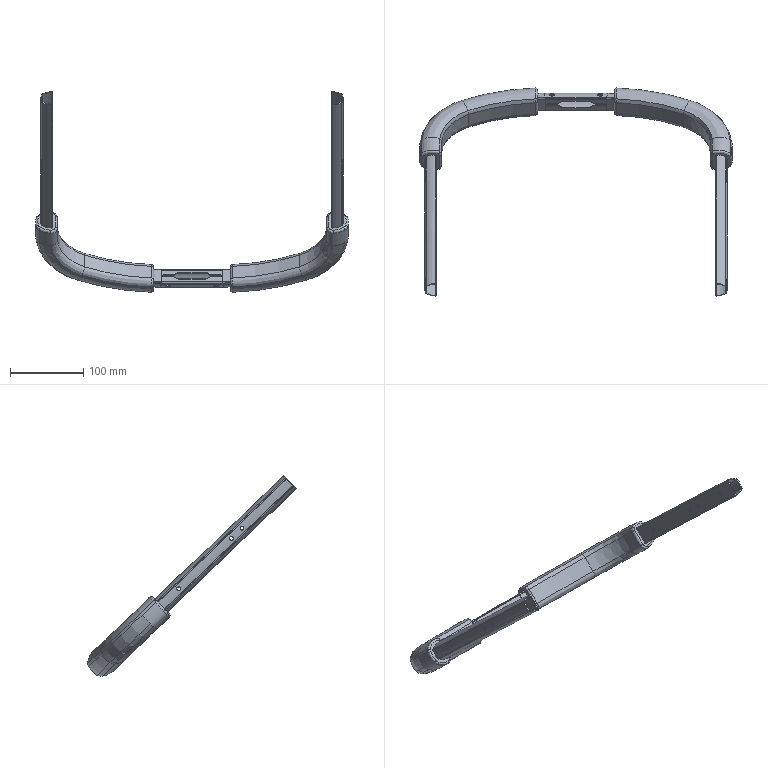Part | SolidWorks | features BaseBody 4 | 3 solids | 359 faces | box 428.555 x 285.247 x 274.529 mm | volume 356846 mm3 | spline 199 | cylinder 140 | plane 20 | commonest cylinder face diameters 5.2 x28 0.6 x21 3 x21 6 x8 7.1 x8 10 x8